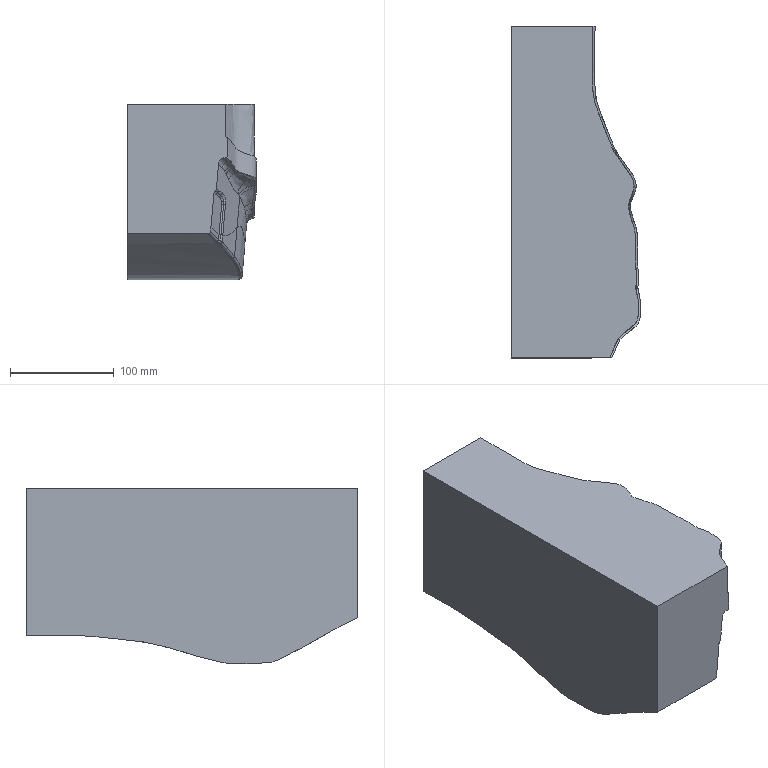Part | NX | features solid 2 | 1 solid | 151 faces | box 124.592 x 320 x 169.264 mm | volume 4806775 mm3 | spline 145 | plane 4 | cylinder 2 | commonest cylinder face diameters 20 x2